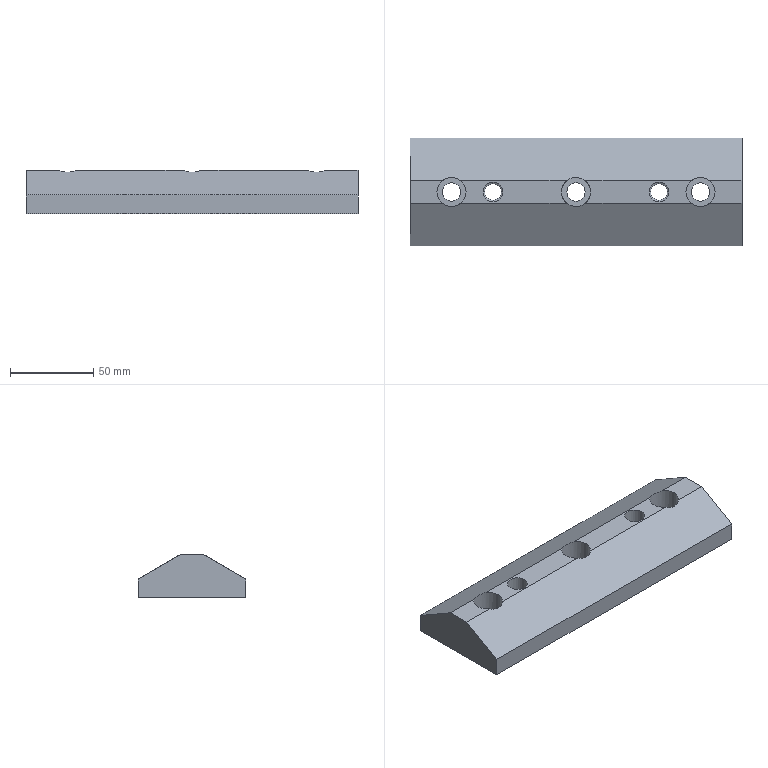Part | NX | features MAIN_BODY 2 | 1 solid | 26 faces | box 200 x 65 x 26 mm | volume 243266 mm3 | plane 14 | cylinder 10 | cone 2 | commonest cylinder face diameters 11 x3 17.5 x3 10 x2 12 x2
STEP:
#1=CARTESIAN_POINT('',(-224.,0.,-139.));
#2=VERTEX_POINT('',#1);
#3=CARTESIAN_POINT('',(-230.,0.,-139.));
#4=DIRECTION('',(0.,0.,1.));
#5=DIRECTION('',(1.,0.,0.));
#6=AXIS2_PLACEMENT_3D('',#3,#4,#5);
#7=CIRCLE('',#6,6.);
#8=EDGE_CURVE('',#2,#2,#7,.T.);
#9=ORIENTED_EDGE('',*,*,#8,.F.);
#10=EDGE_LOOP('',(#9));
#11=FACE_BOUND('',#10,.T.);
#12=CARTESIAN_POINT('',(-249.656,6.928,-139.));
#13=VERTEX_POINT('',#12);
#14=CARTESIAN_POINT('',(-185.344,6.928,-139.));
#15=VERTEX_POINT('',#14);
#16=CARTESIAN_POINT('',(-280.,6.928,-139.));
#17=DIRECTION('',(1.,0.,0.));
#18=VECTOR('',#17,1000.);
#19=LINE('',#16,#18);
#20=EDGE_CURVE('',#13,#15,#19,.T.);
#21=ORIENTED_EDGE('',*,*,#20,.F.);
#22=CARTESIAN_POINT('',(-249.656,-6.928,-139.));
#23=VERTEX_POINT('',#22);
#24=CARTESIAN_POINT('',(-255.,0.,-139.));
#25=DIRECTION('',(0.,0.,1.));
#26=DIRECTION('',(1.,0.,0.));
#27=AXIS2_PLACEMENT_3D('',#24,#25,#26);
#28=CIRCLE('',#27,8.75);
#29=EDGE_CURVE('',#23,#13,#28,.T.);
#30=ORIENTED_EDGE('',*,*,#29,.F.);
#31=CARTESIAN_POINT('',(-185.344,-6.928,-139.));
#32=VERTEX_POINT('',#31);
#33=CARTESIAN_POINT('',(-280.,-6.928,-139.));
#34=DIRECTION('',(1.,0.,0.));
#35=VECTOR('',#34,1000.);
#36=LINE('',#33,#35);
#37=EDGE_CURVE('',#23,#32,#36,.T.);
#38=ORIENTED_EDGE('',*,*,#37,.T.);
#39=CARTESIAN_POINT('',(-180.,0.,-139.));
#40=DIRECTION('',(0.,0.,1.));
#41=DIRECTION('',(1.,0.,0.));
#42=AXIS2_PLACEMENT_3D('',#39,#40,#41);
#43=CIRCLE('',#42,8.75);
#44=EDGE_CURVE('',#15,#32,#43,.T.);
#45=ORIENTED_EDGE('',*,*,#44,.F.);
#46=EDGE_LOOP('',(#21,#30,#38,#45));
#47=FACE_BOUND('',#46,.T.);
#48=CARTESIAN_POINT('',(-80.,32.5,-139.));
#49=DIRECTION('',(0.,0.,-1.));
#50=DIRECTION('',(1.,0.,0.));
#51=AXIS2_PLACEMENT_3D('',#48,#49,#50);
#52=PLANE('',#51);
#53=ADVANCED_FACE('',(#11,#47),#52,.F.);
#54=CARTESIAN_POINT('',(-99.656,6.928,-139.));
#55=VERTEX_POINT('',#54);
#56=CARTESIAN_POINT('',(-80.,6.928,-139.));
#57=VERTEX_POINT('',#56);
#58=CARTESIAN_POINT('',(-280.,6.928,-139.));
#59=DIRECTION('',(1.,0.,0.));
#60=VECTOR('',#59,1000.);
#61=LINE('',#58,#60);
#62=EDGE_CURVE('',#55,#57,#61,.T.);
#63=ORIENTED_EDGE('',*,*,#62,.F.);
#64=CARTESIAN_POINT('',(-99.656,-6.928,-139.));
#65=VERTEX_POINT('',#64);
#66=CARTESIAN_POINT('',(-105.,0.,-139.));
#67=DIRECTION('',(0.,0.,1.));
#68=DIRECTION('',(1.,0.,0.));
#69=AXIS2_PLACEMENT_3D('',#66,#67,#68);
#70=CIRCLE('',#69,8.75);
#71=EDGE_CURVE('',#65,#55,#70,.T.);
#72=ORIENTED_EDGE('',*,*,#71,.F.);
#73=CARTESIAN_POINT('',(-80.,-6.928,-139.));
#74=VERTEX_POINT('',#73);
#75=CARTESIAN_POINT('',(-280.,-6.928,-139.));
#76=DIRECTION('',(1.,0.,0.));
#77=VECTOR('',#76,1000.);
#78=LINE('',#75,#77);
#79=EDGE_CURVE('',#65,#74,#78,.T.);
#80=ORIENTED_EDGE('',*,*,#79,.T.);
#81=CARTESIAN_POINT('',(-80.,32.5,-139.));
#82=DIRECTION('',(0.,-1.,0.));
#83=VECTOR('',#82,1000.);
#84=LINE('',#81,#83);
#85=EDGE_CURVE('',#57,#74,#84,.T.);
#86=ORIENTED_EDGE('',*,*,#85,.F.);
#87=EDGE_LOOP('',(#63,#72,#80,#86));
#88=FACE_BOUND('',#87,.T.);
#89=CARTESIAN_POINT('',(-80.,32.5,-139.));
#90=DIRECTION('',(0.,0.,-1.));
#91=DIRECTION('',(1.,0.,0.));
#92=AXIS2_PLACEMENT_3D('',#89,#90,#91);
#93=PLANE('',#92);
#94=ADVANCED_FACE('',(#88),#93,.F.);
#95=CARTESIAN_POINT('',(-174.656,-6.928,-139.));
#96=VERTEX_POINT('',#95);
#97=CARTESIAN_POINT('',(-110.344,-6.928,-139.));
#98=VERTEX_POINT('',#97);
#99=CARTESIAN_POINT('',(-280.,-6.928,-139.));
#100=DIRECTION('',(1.,0.,0.));
#101=VECTOR('',#100,1000.);
#102=LINE('',#99,#101);
#103=EDGE_CURVE('',#96,#98,#102,.T.);
#104=ORIENTED_EDGE('',*,*,#103,.T.);
#105=CARTESIAN_POINT('',(-110.344,6.928,-139.));
#106=VERTEX_POINT('',#105);
#107=CARTESIAN_POINT('',(-105.,0.,-139.));
#108=DIRECTION('',(0.,0.,1.));
#109=DIRECTION('',(1.,0.,0.));
#110=AXIS2_PLACEMENT_3D('',#107,#108,#109);
#111=CIRCLE('',#110,8.75);
#112=EDGE_CURVE('',#106,#98,#111,.T.);
#113=ORIENTED_EDGE('',*,*,#112,.F.);
#114=CARTESIAN_POINT('',(-174.656,6.928,-139.));
#115=VERTEX_POINT('',#114);
#116=CARTESIAN_POINT('',(-280.,6.928,-139.));
#117=DIRECTION('',(1.,0.,0.));
#118=VECTOR('',#117,1000.);
#119=LINE('',#116,#118);
#120=EDGE_CURVE('',#115,#106,#119,.T.);
#121=ORIENTED_EDGE('',*,*,#120,.F.);
#122=CARTESIAN_POINT('',(-180.,0.,-139.));
#123=DIRECTION('',(0.,0.,1.));
#124=DIRECTION('',(1.,0.,0.));
#125=AXIS2_PLACEMENT_3D('',#122,#123,#124);
#126=CIRCLE('',#125,8.75);
#127=EDGE_CURVE('',#96,#115,#126,.T.);
#128=ORIENTED_EDGE('',*,*,#127,.F.);
#129=EDGE_LOOP('',(#104,#113,#121,#128));
#130=FACE_BOUND('',#129,.T.);
#131=CARTESIAN_POINT('',(-124.,0.,-139.));
#132=VERTEX_POINT('',#131);
#133=CARTESIAN_POINT('',(-130.,0.,-139.));
#134=DIRECTION('',(0.,0.,1.));
#135=DIRECTION('',(1.,0.,0.));
#136=AXIS2_PLACEMENT_3D('',#133,#134,#135);
#137=CIRCLE('',#136,6.);
#138=EDGE_CURVE('',#132,#132,#137,.T.);
#139=ORIENTED_EDGE('',*,*,#138,.F.);
#140=EDGE_LOOP('',(#139));
#141=FACE_BOUND('',#140,.T.);
#142=CARTESIAN_POINT('',(-80.,32.5,-139.));
#143=DIRECTION('',(0.,0.,-1.));
#144=DIRECTION('',(1.,0.,0.));
#145=AXIS2_PLACEMENT_3D('',#142,#143,#144);
#146=PLANE('',#145);
#147=ADVANCED_FACE('',(#130,#141),#146,.F.);
#148=CARTESIAN_POINT('',(-80.,32.5,-153.764));
#149=VERTEX_POINT('',#148);
#150=CARTESIAN_POINT('',(-80.,6.928,-139.));
#151=DIRECTION('',(0.,0.866,-0.5));
#152=VECTOR('',#151,1000.);
#153=LINE('',#150,#152);
#154=EDGE_CURVE('',#57,#149,#153,.T.);
#155=ORIENTED_EDGE('',*,*,#154,.F.);
#156=ORIENTED_EDGE('',*,*,#85,.T.);
#157=CARTESIAN_POINT('',(-80.,-32.5,-153.764));
#158=VERTEX_POINT('',#157);
#159=CARTESIAN_POINT('',(-80.,-32.5,-153.764));
#160=DIRECTION('',(0.,0.866,0.5));
#161=VECTOR('',#160,1000.);
#162=LINE('',#159,#161);
#163=EDGE_CURVE('',#158,#74,#162,.T.);
#164=ORIENTED_EDGE('',*,*,#163,.F.);
#165=CARTESIAN_POINT('',(-80.,-32.5,-165.));
#166=VERTEX_POINT('',#165);
#167=CARTESIAN_POINT('',(-80.,-32.5,-139.));
#168=DIRECTION('',(0.,0.,-1.));
#169=VECTOR('',#168,1000.);
#170=LINE('',#167,#169);
#171=EDGE_CURVE('',#158,#166,#170,.T.);
#172=ORIENTED_EDGE('',*,*,#171,.T.);
#173=CARTESIAN_POINT('',(-80.,32.5,-165.));
#174=VERTEX_POINT('',#173);
#175=CARTESIAN_POINT('',(-80.,32.5,-165.));
#176=DIRECTION('',(0.,-1.,0.));
#177=VECTOR('',#176,1000.);
#178=LINE('',#175,#177);
#179=EDGE_CURVE('',#174,#166,#178,.T.);
#180=ORIENTED_EDGE('',*,*,#179,.F.);
#181=CARTESIAN_POINT('',(-80.,32.5,-139.));
#182=DIRECTION('',(0.,0.,-1.));
#183=VECTOR('',#182,1000.);
#184=LINE('',#181,#183);
#185=EDGE_CURVE('',#149,#174,#184,.T.);
#186=ORIENTED_EDGE('',*,*,#185,.F.);
#187=EDGE_LOOP('',(#155,#156,#164,#172,#180,#186));
#188=FACE_BOUND('',#187,.T.);
#189=CARTESIAN_POINT('',(-80.,32.5,-139.));
#190=DIRECTION('',(-1.,0.,0.));
#191=DIRECTION('',(0.,1.,0.));
#192=AXIS2_PLACEMENT_3D('',#189,#190,#191);
#193=PLANE('',#192);
#194=ADVANCED_FACE('',(#188),#193,.F.);
#195=CARTESIAN_POINT('',(-280.,-32.5,-153.764));
#196=VERTEX_POINT('',#195);
#197=CARTESIAN_POINT('',(-280.,-32.5,-153.764));
#198=DIRECTION('',(1.,0.,0.));
#199=VECTOR('',#198,1000.);
#200=LINE('',#197,#199);
#201=EDGE_CURVE('',#196,#158,#200,.T.);
#202=ORIENTED_EDGE('',*,*,#201,.F.);
#203=CARTESIAN_POINT('',(-280.,-32.5,-165.));
#204=VERTEX_POINT('',#203);
#205=CARTESIAN_POINT('',(-280.,-32.5,-139.));
#206=DIRECTION('',(0.,0.,-1.));
#207=VECTOR('',#206,1000.);
#208=LINE('',#205,#207);
#209=EDGE_CURVE('',#196,#204,#208,.T.);
#210=ORIENTED_EDGE('',*,*,#209,.T.);
#211=CARTESIAN_POINT('',(-80.,-32.5,-165.));
#212=DIRECTION('',(-1.,0.,0.));
#213=VECTOR('',#212,1000.);
#214=LINE('',#211,#213);
#215=EDGE_CURVE('',#166,#204,#214,.T.);
#216=ORIENTED_EDGE('',*,*,#215,.F.);
#217=ORIENTED_EDGE('',*,*,#171,.F.);
#218=EDGE_LOOP('',(#202,#210,#216,#217));
#219=FACE_BOUND('',#218,.T.);
#220=CARTESIAN_POINT('',(-80.,-32.5,-139.));
#221=DIRECTION('',(0.,1.,0.));
#222=DIRECTION('',(1.,0.,0.));
#223=AXIS2_PLACEMENT_3D('',#220,#221,#222);
#224=PLANE('',#223);
#225=ADVANCED_FACE('',(#219),#224,.F.);
#226=CARTESIAN_POINT('',(-280.,6.928,-139.));
#227=VERTEX_POINT('',#226);
#228=CARTESIAN_POINT('',(-280.,32.5,-153.764));
#229=VERTEX_POINT('',#228);
#230=CARTESIAN_POINT('',(-280.,6.928,-139.));
#231=DIRECTION('',(0.,0.866,-0.5));
#232=VECTOR('',#231,1000.);
#233=LINE('',#230,#232);
#234=EDGE_CURVE('',#227,#229,#233,.T.);
#235=ORIENTED_EDGE('',*,*,#234,.T.);
#236=CARTESIAN_POINT('',(-280.,32.5,-165.));
#237=VERTEX_POINT('',#236);
#238=CARTESIAN_POINT('',(-280.,32.5,-139.));
#239=DIRECTION('',(0.,0.,-1.));
#240=VECTOR('',#239,1000.);
#241=LINE('',#238,#240);
#242=EDGE_CURVE('',#229,#237,#241,.T.);
#243=ORIENTED_EDGE('',*,*,#242,.T.);
#244=CARTESIAN_POINT('',(-280.,-32.5,-165.));
#245=DIRECTION('',(0.,1.,0.));
#246=VECTOR('',#245,1000.);
#247=LINE('',#244,#246);
#248=EDGE_CURVE('',#204,#237,#247,.T.);
#249=ORIENTED_EDGE('',*,*,#248,.F.);
#250=ORIENTED_EDGE('',*,*,#209,.F.);
#251=CARTESIAN_POINT('',(-280.,-6.928,-139.));
#252=VERTEX_POINT('',#251);
#253=CARTESIAN_POINT('',(-280.,-32.5,-153.764));
#254=DIRECTION('',(0.,0.866,0.5));
#255=VECTOR('',#254,1000.);
#256=LINE('',#253,#255);
#257=EDGE_CURVE('',#196,#252,#256,.T.);
#258=ORIENTED_EDGE('',*,*,#257,.T.);
#259=CARTESIAN_POINT('',(-280.,-32.5,-139.));
#260=DIRECTION('',(0.,1.,0.));
#261=VECTOR('',#260,1000.);
#262=LINE('',#259,#261);
#263=EDGE_CURVE('',#252,#227,#262,.T.);
#264=ORIENTED_EDGE('',*,*,#263,.T.);
#265=EDGE_LOOP('',(#235,#243,#249,#250,#258,#264));
#266=FACE_BOUND('',#265,.T.);
#267=CARTESIAN_POINT('',(-280.,-32.5,-139.));
#268=DIRECTION('',(1.,0.,0.));
#269=DIRECTION('',(0.,0.,1.));
#270=AXIS2_PLACEMENT_3D('',#267,#268,#269);
#271=PLANE('',#270);
#272=ADVANCED_FACE('',(#266),#271,.F.);
#273=CARTESIAN_POINT('',(-280.,32.5,-153.764));
#274=DIRECTION('',(1.,0.,0.));
#275=VECTOR('',#274,1000.);
#276=LINE('',#273,#275);
#277=EDGE_CURVE('',#229,#149,#276,.T.);
#278=ORIENTED_EDGE('',*,*,#277,.T.);
#279=ORIENTED_EDGE('',*,*,#185,.T.);
#280=CARTESIAN_POINT('',(-280.,32.5,-165.));
#281=DIRECTION('',(1.,0.,0.));
#282=VECTOR('',#281,1000.);
#283=LINE('',#280,#282);
#284=EDGE_CURVE('',#237,#174,#283,.T.);
#285=ORIENTED_EDGE('',*,*,#284,.F.);
#286=ORIENTED_EDGE('',*,*,#242,.F.);
#287=EDGE_LOOP('',(#278,#279,#285,#286));
#288=FACE_BOUND('',#287,.T.);
#289=CARTESIAN_POINT('',(-280.,32.5,-139.));
#290=DIRECTION('',(0.,-1.,0.));
#291=DIRECTION('',(0.,0.,-1.));
#292=AXIS2_PLACEMENT_3D('',#289,#290,#291);
#293=PLANE('',#292);
#294=ADVANCED_FACE('',(#288),#293,.F.);
#295=CARTESIAN_POINT('',(-260.344,6.928,-139.));
#296=VERTEX_POINT('',#295);
#297=CARTESIAN_POINT('',(-280.,6.928,-139.));
#298=DIRECTION('',(1.,0.,0.));
#299=VECTOR('',#298,1000.);
#300=LINE('',#297,#299);
#301=EDGE_CURVE('',#227,#296,#300,.T.);
#302=ORIENTED_EDGE('',*,*,#301,.F.);
#303=ORIENTED_EDGE('',*,*,#263,.F.);
#304=CARTESIAN_POINT('',(-260.344,-6.928,-139.));
#305=VERTEX_POINT('',#304);
#306=CARTESIAN_POINT('',(-280.,-6.928,-139.));
#307=DIRECTION('',(1.,0.,0.));
#308=VECTOR('',#307,1000.);
#309=LINE('',#306,#308);
#310=EDGE_CURVE('',#252,#305,#309,.T.);
#311=ORIENTED_EDGE('',*,*,#310,.T.);
#312=CARTESIAN_POINT('',(-255.,0.,-139.));
#313=DIRECTION('',(0.,0.,1.));
#314=DIRECTION('',(1.,0.,0.));
#315=AXIS2_PLACEMENT_3D('',#312,#313,#314);
#316=CIRCLE('',#315,8.75);
#317=EDGE_CURVE('',#296,#305,#316,.T.);
#318=ORIENTED_EDGE('',*,*,#317,.F.);
#319=EDGE_LOOP('',(#302,#303,#311,#318));
#320=FACE_BOUND('',#319,.T.);
#321=CARTESIAN_POINT('',(-80.,32.5,-139.));
#322=DIRECTION('',(0.,0.,-1.));
#323=DIRECTION('',(1.,0.,0.));
#324=AXIS2_PLACEMENT_3D('',#321,#322,#323);
#325=PLANE('',#324);
#326=ADVANCED_FACE('',(#320),#325,.F.);
#327=CARTESIAN_POINT('',(-174.5,0.,-165.));
#328=VERTEX_POINT('',#327);
#329=CARTESIAN_POINT('',(-180.,0.,-165.));
#330=DIRECTION('',(0.,0.,1.));
#331=DIRECTION('',(1.,0.,0.));
#332=AXIS2_PLACEMENT_3D('',#329,#330,#331);
#333=CIRCLE('',#332,5.5);
#334=EDGE_CURVE('',#328,#328,#333,.T.);
#335=ORIENTED_EDGE('',*,*,#334,.T.);
#336=EDGE_LOOP('',(#335));
#337=FACE_BOUND('',#336,.T.);
#338=CARTESIAN_POINT('',(-235.,0.,-165.));
#339=VERTEX_POINT('',#338);
#340=CARTESIAN_POINT('',(-230.,0.,-165.));
#341=DIRECTION('',(0.,0.,-1.));
#342=DIRECTION('',(-1.,0.,0.));
#343=AXIS2_PLACEMENT_3D('',#340,#341,#342);
#344=CIRCLE('',#343,5.);
#345=EDGE_CURVE('',#339,#339,#344,.T.);
#346=ORIENTED_EDGE('',*,*,#345,.F.);
#347=EDGE_LOOP('',(#346));
#348=FACE_BOUND('',#347,.T.);
#349=CARTESIAN_POINT('',(-135.,0.,-165.));
#350=VERTEX_POINT('',#349);
#351=CARTESIAN_POINT('',(-130.,0.,-165.));
#352=DIRECTION('',(0.,0.,-1.));
#353=DIRECTION('',(-1.,0.,0.));
#354=AXIS2_PLACEMENT_3D('',#351,#352,#353);
#355=CIRCLE('',#354,5.);
#356=EDGE_CURVE('',#350,#350,#355,.T.);
#357=ORIENTED_EDGE('',*,*,#356,.F.);
#358=EDGE_LOOP('',(#357));
#359=FACE_BOUND('',#358,.T.);
#360=CARTESIAN_POINT('',(-249.5,0.,-165.));
#361=VERTEX_POINT('',#360);
#362=CARTESIAN_POINT('',(-255.,0.,-165.));
#363=DIRECTION('',(0.,0.,1.));
#364=DIRECTION('',(1.,0.,0.));
#365=AXIS2_PLACEMENT_3D('',#362,#363,#364);
#366=CIRCLE('',#365,5.5);
#367=EDGE_CURVE('',#361,#361,#366,.T.);
#368=ORIENTED_EDGE('',*,*,#367,.T.);
#369=EDGE_LOOP('',(#368));
#370=FACE_BOUND('',#369,.T.);
#371=CARTESIAN_POINT('',(-99.5,0.,-165.));
#372=VERTEX_POINT('',#371);
#373=CARTESIAN_POINT('',(-105.,0.,-165.));
#374=DIRECTION('',(0.,0.,1.));
#375=DIRECTION('',(1.,0.,0.));
#376=AXIS2_PLACEMENT_3D('',#373,#374,#375);
#377=CIRCLE('',#376,5.5);
#378=EDGE_CURVE('',#372,#372,#377,.T.);
#379=ORIENTED_EDGE('',*,*,#378,.T.);
#380=EDGE_LOOP('',(#379));
#381=FACE_BOUND('',#380,.T.);
#382=ORIENTED_EDGE('',*,*,#179,.T.);
#383=ORIENTED_EDGE('',*,*,#215,.T.);
#384=ORIENTED_EDGE('',*,*,#248,.T.);
#385=ORIENTED_EDGE('',*,*,#284,.T.);
#386=EDGE_LOOP('',(#382,#383,#384,#385));
#387=FACE_BOUND('',#386,.T.);
#388=CARTESIAN_POINT('',(-80.,32.5,-165.));
#389=DIRECTION('',(0.,0.,-1.));
#390=DIRECTION('',(1.,0.,0.));
#391=AXIS2_PLACEMENT_3D('',#388,#389,#390);
#392=PLANE('',#391);
#393=ADVANCED_FACE('',(#337,#348,#359,#370,#381,#387),#392,.T.);
#394=ORIENTED_EDGE('',*,*,#378,.F.);
#395=EDGE_LOOP('',(#394));
#396=FACE_BOUND('',#395,.T.);
#397=CARTESIAN_POINT('',(-99.5,0.,-155.));
#398=VERTEX_POINT('',#397);
#399=CARTESIAN_POINT('',(-105.,0.,-155.));
#400=DIRECTION('',(0.,0.,1.));
#401=DIRECTION('',(1.,0.,0.));
#402=AXIS2_PLACEMENT_3D('',#399,#400,#401);
#403=CIRCLE('',#402,5.5);
#404=EDGE_CURVE('',#398,#398,#403,.T.);
#405=ORIENTED_EDGE('',*,*,#404,.T.);
#406=EDGE_LOOP('',(#405));
#407=FACE_BOUND('',#406,.T.);
#408=CARTESIAN_POINT('',(-105.,0.,-165.));
#409=DIRECTION('',(0.,0.,-1.));
#410=DIRECTION('',(1.,0.,0.));
#411=AXIS2_PLACEMENT_3D('',#408,#409,#410);
#412=CYLINDRICAL_SURFACE('',#411,5.5);
#413=ADVANCED_FACE('',(#396,#407),#412,.F.);
#414=ORIENTED_EDGE('',*,*,#404,.F.);
#415=EDGE_LOOP('',(#414));
#416=FACE_BOUND('',#415,.T.);
#417=CARTESIAN_POINT('',(-96.25,0.,-155.));
#418=VERTEX_POINT('',#417);
#419=CARTESIAN_POINT('',(-105.,0.,-155.));
#420=DIRECTION('',(0.,0.,1.));
#421=DIRECTION('',(1.,0.,0.));
#422=AXIS2_PLACEMENT_3D('',#419,#420,#421);
#423=CIRCLE('',#422,8.75);
#424=EDGE_CURVE('',#418,#418,#423,.T.);
#425=ORIENTED_EDGE('',*,*,#424,.T.);
#426=EDGE_LOOP('',(#425));
#427=FACE_BOUND('',#426,.T.);
#428=CARTESIAN_POINT('',(-105.,0.,-155.));
#429=DIRECTION('',(0.,0.,-1.));
#430=DIRECTION('',(1.,0.,0.));
#431=AXIS2_PLACEMENT_3D('',#428,#429,#430);
#432=PLANE('',#431);
#433=ADVANCED_FACE('',(#416,#427),#432,.F.);
#434=CARTESIAN_POINT('',(-105.,0.,-135.));
#435=DIRECTION('',(0.,-0.5,-0.866));
#436=DIRECTION('',(0.,0.866,-0.5));
#437=AXIS2_PLACEMENT_3D('',#434,#435,#436);
#438=ELLIPSE('',#437,10.104,8.75);
#439=EDGE_CURVE('',#55,#106,#438,.F.);
#440=ORIENTED_EDGE('',*,*,#439,.T.);
#441=ORIENTED_EDGE('',*,*,#112,.T.);
#442=CARTESIAN_POINT('',(-105.,0.,-135.));
#443=DIRECTION('',(0.,0.5,-0.866));
#444=DIRECTION('',(0.,-0.866,-0.5));
#445=AXIS2_PLACEMENT_3D('',#442,#443,#444);
#446=ELLIPSE('',#445,10.104,8.75);
#447=EDGE_CURVE('',#98,#65,#446,.F.);
#448=ORIENTED_EDGE('',*,*,#447,.T.);
#449=ORIENTED_EDGE('',*,*,#71,.T.);
#450=EDGE_LOOP('',(#440,#441,#448,#449));
#451=FACE_BOUND('',#450,.T.);
#452=ORIENTED_EDGE('',*,*,#424,.F.);
#453=EDGE_LOOP('',(#452));
#454=FACE_BOUND('',#453,.T.);
#455=CARTESIAN_POINT('',(-105.,0.,-139.));
#456=DIRECTION('',(0.,0.,-1.));
#457=DIRECTION('',(1.,0.,0.));
#458=AXIS2_PLACEMENT_3D('',#455,#456,#457);
#459=CYLINDRICAL_SURFACE('',#458,8.75);
#460=ADVANCED_FACE('',(#451,#454),#459,.F.);
#461=ORIENTED_EDGE('',*,*,#367,.F.);
#462=EDGE_LOOP('',(#461));
#463=FACE_BOUND('',#462,.T.);
#464=CARTESIAN_POINT('',(-249.5,0.,-155.));
#465=VERTEX_POINT('',#464);
#466=CARTESIAN_POINT('',(-255.,0.,-155.));
#467=DIRECTION('',(0.,0.,1.));
#468=DIRECTION('',(1.,0.,0.));
#469=AXIS2_PLACEMENT_3D('',#466,#467,#468);
#470=CIRCLE('',#469,5.5);
#471=EDGE_CURVE('',#465,#465,#470,.T.);
#472=ORIENTED_EDGE('',*,*,#471,.T.);
#473=EDGE_LOOP('',(#472));
#474=FACE_BOUND('',#473,.T.);
#475=CARTESIAN_POINT('',(-255.,0.,-165.));
#476=DIRECTION('',(0.,0.,-1.));
#477=DIRECTION('',(1.,0.,0.));
#478=AXIS2_PLACEMENT_3D('',#475,#476,#477);
#479=CYLINDRICAL_SURFACE('',#478,5.5);
#480=ADVANCED_FACE('',(#463,#474),#479,.F.);
#481=ORIENTED_EDGE('',*,*,#471,.F.);
#482=EDGE_LOOP('',(#481));
#483=FACE_BOUND('',#482,.T.);
#484=CARTESIAN_POINT('',(-246.25,0.,-155.));
#485=VERTEX_POINT('',#484);
#486=CARTESIAN_POINT('',(-255.,0.,-155.));
#487=DIRECTION('',(0.,0.,1.));
#488=DIRECTION('',(1.,0.,0.));
#489=AXIS2_PLACEMENT_3D('',#486,#487,#488);
#490=CIRCLE('',#489,8.75);
#491=EDGE_CURVE('',#485,#485,#490,.T.);
#492=ORIENTED_EDGE('',*,*,#491,.T.);
#493=EDGE_LOOP('',(#492));
#494=FACE_BOUND('',#493,.T.);
#495=CARTESIAN_POINT('',(-255.,0.,-155.));
#496=DIRECTION('',(0.,0.,-1.));
#497=DIRECTION('',(1.,0.,0.));
#498=AXIS2_PLACEMENT_3D('',#495,#496,#497);
#499=PLANE('',#498);
#500=ADVANCED_FACE('',(#483,#494),#499,.F.);
#501=CARTESIAN_POINT('',(-255.,0.,-135.));
#502=DIRECTION('',(0.,-0.5,-0.866));
#503=DIRECTION('',(0.,0.866,-0.5));
#504=AXIS2_PLACEMENT_3D('',#501,#502,#503);
#505=ELLIPSE('',#504,10.104,8.75);
#506=EDGE_CURVE('',#13,#296,#505,.F.);
#507=ORIENTED_EDGE('',*,*,#506,.T.);
#508=ORIENTED_EDGE('',*,*,#317,.T.);
#509=CARTESIAN_POINT('',(-255.,0.,-135.));
#510=DIRECTION('',(0.,0.5,-0.866));
#511=DIRECTION('',(0.,-0.866,-0.5));
#512=AXIS2_PLACEMENT_3D('',#509,#510,#511);
#513=ELLIPSE('',#512,10.104,8.75);
#514=EDGE_CURVE('',#305,#23,#513,.F.);
#515=ORIENTED_EDGE('',*,*,#514,.T.);
#516=ORIENTED_EDGE('',*,*,#29,.T.);
#517=EDGE_LOOP('',(#507,#508,#515,#516));
#518=FACE_BOUND('',#517,.T.);
#519=ORIENTED_EDGE('',*,*,#491,.F.);
#520=EDGE_LOOP('',(#519));
#521=FACE_BOUND('',#520,.T.);
#522=CARTESIAN_POINT('',(-255.,0.,-139.));
#523=DIRECTION('',(0.,0.,-1.));
#524=DIRECTION('',(1.,0.,0.));
#525=AXIS2_PLACEMENT_3D('',#522,#523,#524);
#526=CYLINDRICAL_SURFACE('',#525,8.75);
#527=ADVANCED_FACE('',(#518,#521),#526,.F.);
#528=CARTESIAN_POINT('',(-135.,0.,-150.577));
#529=VERTEX_POINT('',#528);
#530=CARTESIAN_POINT('',(-130.,0.,-150.577));
#531=DIRECTION('',(0.,0.,-1.));
#532=DIRECTION('',(-1.,0.,0.));
#533=AXIS2_PLACEMENT_3D('',#530,#531,#532);
#534=CIRCLE('',#533,5.);
#535=EDGE_CURVE('',#529,#529,#534,.F.);
#536=ORIENTED_EDGE('',*,*,#535,.F.);
#537=EDGE_LOOP('',(#536));
#538=FACE_BOUND('',#537,.T.);
#539=CARTESIAN_POINT('',(-124.,0.,-150.));
#540=VERTEX_POINT('',#539);
#541=CARTESIAN_POINT('',(-130.,0.,-150.));
#542=DIRECTION('',(0.,0.,1.));
#543=DIRECTION('',(1.,0.,0.));
#544=AXIS2_PLACEMENT_3D('',#541,#542,#543);
#545=CIRCLE('',#544,6.);
#546=EDGE_CURVE('',#540,#540,#545,.T.);
#547=ORIENTED_EDGE('',*,*,#546,.T.);
#548=EDGE_LOOP('',(#547));
#549=FACE_BOUND('',#548,.T.);
#550=CARTESIAN_POINT('',(-130.,0.,-150.));
#551=DIRECTION('',(0.,0.,1.));
#552=DIRECTION('',(-1.,0.,0.));
#553=AXIS2_PLACEMENT_3D('',#550,#551,#552);
#554=CONICAL_SURFACE('',#553,6.,1.047);
#555=ADVANCED_FACE('',(#538,#549),#554,.F.);
#556=ORIENTED_EDGE('',*,*,#546,.F.);
#557=EDGE_LOOP('',(#556));
#558=FACE_BOUND('',#557,.T.);
#559=ORIENTED_EDGE('',*,*,#138,.T.);
#560=EDGE_LOOP('',(#559));
#561=FACE_BOUND('',#560,.T.);
#562=CARTESIAN_POINT('',(-130.,0.,-139.));
#563=DIRECTION('',(0.,0.,-1.));
#564=DIRECTION('',(1.,0.,0.));
#565=AXIS2_PLACEMENT_3D('',#562,#563,#564);
#566=CYLINDRICAL_SURFACE('',#565,6.);
#567=ADVANCED_FACE('',(#558,#561),#566,.F.);
#568=CARTESIAN_POINT('',(-235.,0.,-150.577));
#569=VERTEX_POINT('',#568);
#570=CARTESIAN_POINT('',(-230.,0.,-150.577));
#571=DIRECTION('',(0.,0.,-1.));
#572=DIRECTION('',(-1.,0.,0.));
#573=AXIS2_PLACEMENT_3D('',#570,#571,#572);
#574=CIRCLE('',#573,5.);
#575=EDGE_CURVE('',#569,#569,#574,.F.);
#576=ORIENTED_EDGE('',*,*,#575,.F.);
#577=EDGE_LOOP('',(#576));
#578=FACE_BOUND('',#577,.T.);
#579=CARTESIAN_POINT('',(-224.,0.,-150.));
#580=VERTEX_POINT('',#579);
#581=CARTESIAN_POINT('',(-230.,0.,-150.));
#582=DIRECTION('',(0.,0.,1.));
#583=DIRECTION('',(1.,0.,0.));
#584=AXIS2_PLACEMENT_3D('',#581,#582,#583);
#585=CIRCLE('',#584,6.);
#586=EDGE_CURVE('',#580,#580,#585,.T.);
#587=ORIENTED_EDGE('',*,*,#586,.T.);
#588=EDGE_LOOP('',(#587));
#589=FACE_BOUND('',#588,.T.);
#590=CARTESIAN_POINT('',(-230.,0.,-150.));
#591=DIRECTION('',(0.,0.,1.));
#592=DIRECTION('',(-1.,0.,0.));
#593=AXIS2_PLACEMENT_3D('',#590,#591,#592);
#594=CONICAL_SURFACE('',#593,6.,1.047);
#595=ADVANCED_FACE('',(#578,#589),#594,.F.);
#596=ORIENTED_EDGE('',*,*,#586,.F.);
#597=EDGE_LOOP('',(#596));
#598=FACE_BOUND('',#597,.T.);
#599=ORIENTED_EDGE('',*,*,#8,.T.);
#600=EDGE_LOOP('',(#599));
#601=FACE_BOUND('',#600,.T.);
#602=CARTESIAN_POINT('',(-230.,0.,-139.));
#603=DIRECTION('',(0.,0.,-1.));
#604=DIRECTION('',(1.,0.,0.));
#605=AXIS2_PLACEMENT_3D('',#602,#603,#604);
#606=CYLINDRICAL_SURFACE('',#605,6.);
#607=ADVANCED_FACE('',(#598,#601),#606,.F.);
#608=ORIENTED_EDGE('',*,*,#356,.T.);
#609=EDGE_LOOP('',(#608));
#610=FACE_BOUND('',#609,.T.);
#611=ORIENTED_EDGE('',*,*,#535,.T.);
#612=EDGE_LOOP('',(#611));
#613=FACE_BOUND('',#612,.T.);
#614=CARTESIAN_POINT('',(-130.,0.,-165.));
#615=DIRECTION('',(0.,0.,1.));
#616=DIRECTION('',(-1.,0.,0.));
#617=AXIS2_PLACEMENT_3D('',#614,#615,#616);
#618=CYLINDRICAL_SURFACE('',#617,5.);
#619=ADVANCED_FACE('',(#610,#613),#618,.F.);
#620=ORIENTED_EDGE('',*,*,#345,.T.);
#621=EDGE_LOOP('',(#620));
#622=FACE_BOUND('',#621,.T.);
#623=ORIENTED_EDGE('',*,*,#575,.T.);
#624=EDGE_LOOP('',(#623));
#625=FACE_BOUND('',#624,.T.);
#626=CARTESIAN_POINT('',(-230.,0.,-165.));
#627=DIRECTION('',(0.,0.,1.));
#628=DIRECTION('',(-1.,0.,0.));
#629=AXIS2_PLACEMENT_3D('',#626,#627,#628);
#630=CYLINDRICAL_SURFACE('',#629,5.);
#631=ADVANCED_FACE('',(#622,#625),#630,.F.);
#632=CARTESIAN_POINT('',(-180.,0.,-135.));
#633=DIRECTION('',(0.,0.5,-0.866));
#634=DIRECTION('',(0.,-0.866,-0.5));
#635=AXIS2_PLACEMENT_3D('',#632,#633,#634);
#636=ELLIPSE('',#635,10.104,8.75);
#637=EDGE_CURVE('',#96,#32,#636,.T.);
#638=ORIENTED_EDGE('',*,*,#637,.T.);
#639=ORIENTED_EDGE('',*,*,#37,.F.);
#640=ORIENTED_EDGE('',*,*,#514,.F.);
#641=ORIENTED_EDGE('',*,*,#310,.F.);
#642=ORIENTED_EDGE('',*,*,#257,.F.);
#643=ORIENTED_EDGE('',*,*,#201,.T.);
#644=ORIENTED_EDGE('',*,*,#163,.T.);
#645=ORIENTED_EDGE('',*,*,#79,.F.);
#646=ORIENTED_EDGE('',*,*,#447,.F.);
#647=ORIENTED_EDGE('',*,*,#103,.F.);
#648=EDGE_LOOP('',(#638,#639,#640,#641,#642,#643,#644,#645,#646,#647));
#649=FACE_BOUND('',#648,.T.);
#650=CARTESIAN_POINT('',(-280.,-32.5,-153.764));
#651=DIRECTION('',(0.,-0.5,0.866));
#652=DIRECTION('',(0.,-0.866,-0.5));
#653=AXIS2_PLACEMENT_3D('',#650,#651,#652);
#654=PLANE('',#653);
#655=ADVANCED_FACE('',(#649),#654,.T.);
#656=CARTESIAN_POINT('',(-180.,0.,-135.));
#657=DIRECTION('',(0.,-0.5,-0.866));
#658=DIRECTION('',(0.,0.866,-0.5));
#659=AXIS2_PLACEMENT_3D('',#656,#657,#658);
#660=ELLIPSE('',#659,10.104,8.75);
#661=EDGE_CURVE('',#15,#115,#660,.T.);
#662=ORIENTED_EDGE('',*,*,#661,.T.);
#663=ORIENTED_EDGE('',*,*,#120,.T.);
#664=ORIENTED_EDGE('',*,*,#439,.F.);
#665=ORIENTED_EDGE('',*,*,#62,.T.);
#666=ORIENTED_EDGE('',*,*,#154,.T.);
#667=ORIENTED_EDGE('',*,*,#277,.F.);
#668=ORIENTED_EDGE('',*,*,#234,.F.);
#669=ORIENTED_EDGE('',*,*,#301,.T.);
#670=ORIENTED_EDGE('',*,*,#506,.F.);
#671=ORIENTED_EDGE('',*,*,#20,.T.);
#672=EDGE_LOOP('',(#662,#663,#664,#665,#666,#667,#668,#669,#670,#671));
#673=FACE_BOUND('',#672,.T.);
#674=CARTESIAN_POINT('',(-280.,6.928,-139.));
#675=DIRECTION('',(0.,0.5,0.866));
#676=DIRECTION('',(0.,-0.866,0.5));
#677=AXIS2_PLACEMENT_3D('',#674,#675,#676);
#678=PLANE('',#677);
#679=ADVANCED_FACE('',(#673),#678,.T.);
#680=ORIENTED_EDGE('',*,*,#334,.F.);
#681=EDGE_LOOP('',(#680));
#682=FACE_BOUND('',#681,.T.);
#683=CARTESIAN_POINT('',(-174.5,0.,-155.));
#684=VERTEX_POINT('',#683);
#685=CARTESIAN_POINT('',(-180.,0.,-155.));
#686=DIRECTION('',(0.,0.,1.));
#687=DIRECTION('',(1.,0.,0.));
#688=AXIS2_PLACEMENT_3D('',#685,#686,#687);
#689=CIRCLE('',#688,5.5);
#690=EDGE_CURVE('',#684,#684,#689,.T.);
#691=ORIENTED_EDGE('',*,*,#690,.T.);
#692=EDGE_LOOP('',(#691));
#693=FACE_BOUND('',#692,.T.);
#694=CARTESIAN_POINT('',(-180.,0.,-165.));
#695=DIRECTION('',(0.,0.,-1.));
#696=DIRECTION('',(1.,0.,0.));
#697=AXIS2_PLACEMENT_3D('',#694,#695,#696);
#698=CYLINDRICAL_SURFACE('',#697,5.5);
#699=ADVANCED_FACE('',(#682,#693),#698,.F.);
#700=ORIENTED_EDGE('',*,*,#690,.F.);
#701=EDGE_LOOP('',(#700));
#702=FACE_BOUND('',#701,.T.);
#703=CARTESIAN_POINT('',(-171.25,0.,-155.));
#704=VERTEX_POINT('',#703);
#705=CARTESIAN_POINT('',(-180.,0.,-155.));
#706=DIRECTION('',(0.,0.,1.));
#707=DIRECTION('',(1.,0.,0.));
#708=AXIS2_PLACEMENT_3D('',#705,#706,#707);
#709=CIRCLE('',#708,8.75);
#710=EDGE_CURVE('',#704,#704,#709,.T.);
#711=ORIENTED_EDGE('',*,*,#710,.T.);
#712=EDGE_LOOP('',(#711));
#713=FACE_BOUND('',#712,.T.);
#714=CARTESIAN_POINT('',(-180.,0.,-155.));
#715=DIRECTION('',(0.,0.,-1.));
#716=DIRECTION('',(1.,0.,0.));
#717=AXIS2_PLACEMENT_3D('',#714,#715,#716);
#718=PLANE('',#717);
#719=ADVANCED_FACE('',(#702,#713),#718,.F.);
#720=ORIENTED_EDGE('',*,*,#637,.F.);
#721=ORIENTED_EDGE('',*,*,#127,.T.);
#722=ORIENTED_EDGE('',*,*,#661,.F.);
#723=ORIENTED_EDGE('',*,*,#44,.T.);
#724=EDGE_LOOP('',(#720,#721,#722,#723));
#725=FACE_BOUND('',#724,.T.);
#726=ORIENTED_EDGE('',*,*,#710,.F.);
#727=EDGE_LOOP('',(#726));
#728=FACE_BOUND('',#727,.T.);
#729=CARTESIAN_POINT('',(-180.,0.,-139.));
#730=DIRECTION('',(0.,0.,-1.));
#731=DIRECTION('',(1.,0.,0.));
#732=AXIS2_PLACEMENT_3D('',#729,#730,#731);
#733=CYLINDRICAL_SURFACE('',#732,8.75);
#734=ADVANCED_FACE('',(#725,#728),#733,.F.);
#735=CLOSED_SHELL('',(#53,#94,#147,#194,#225,#272,#294,#326,#393,#413,#433,#460,#480,#500,#527,#555,#567,#595,#607,#619,#631,#655,#679,#699,#719,#734));
#736=MANIFOLD_SOLID_BREP('',#735);
#737=(LENGTH_UNIT()NAMED_UNIT(*)SI_UNIT(.MILLI.,.METRE.));
#738=UNCERTAINTY_MEASURE_WITH_UNIT(LENGTH_MEASURE(0.00001),#737,'','');
#739=(NAMED_UNIT(*)PLANE_ANGLE_UNIT()SI_UNIT($,.RADIAN.));
#740=(NAMED_UNIT(*)SI_UNIT($,.STERADIAN.)SOLID_ANGLE_UNIT());
#741=(GEOMETRIC_REPRESENTATION_CONTEXT(3)GLOBAL_UNCERTAINTY_ASSIGNED_CONTEXT((#738))GLOBAL_UNIT_ASSIGNED_CONTEXT((#737,#739,#740))REPRESENTATION_CONTEXT('',''));
#742=ADVANCED_BREP_SHAPE_REPRESENTATION('',(#736),#741);